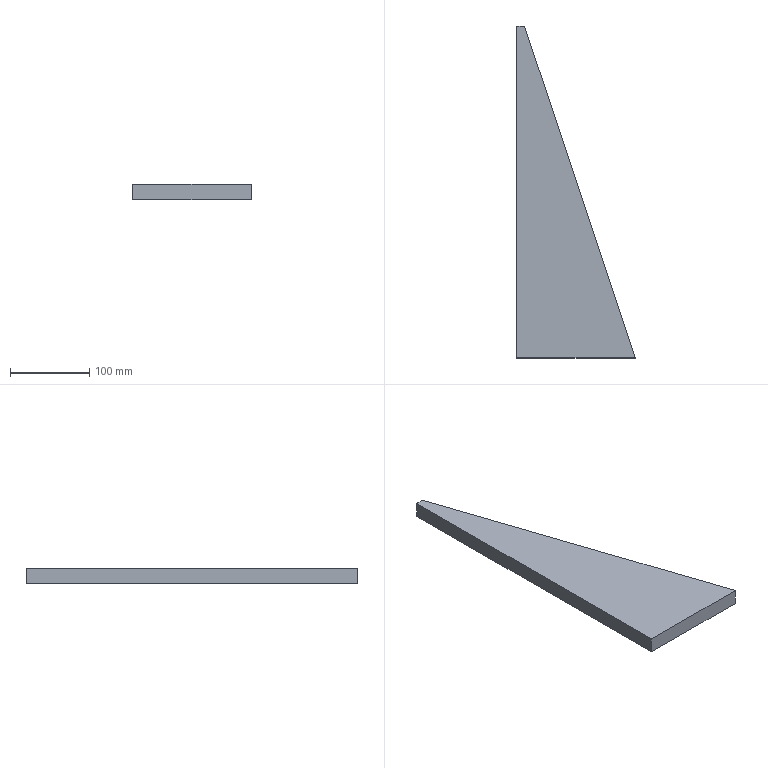Part | SolidWorks | features Extrusion 1 | 1 solid | 6 faces | box 150 x 420 x 20 mm | volume 672000 mm3 | plane 6
STEP:
#1=CARTESIAN_POINT('',(0.,420.,0.));
#2=VERTEX_POINT('',#1);
#3=CARTESIAN_POINT('',(0.,0.,0.));
#4=VERTEX_POINT('',#3);
#5=CARTESIAN_POINT('',(0.,0.,0.));
#6=DIRECTION('',(0.,-1.,0.));
#7=VECTOR('',#6,1000.);
#8=LINE('',#5,#7);
#9=EDGE_CURVE('',#2,#4,#8,.T.);
#10=ORIENTED_EDGE('',*,*,#9,.T.);
#11=CARTESIAN_POINT('',(0.,0.,20.));
#12=VERTEX_POINT('',#11);
#13=CARTESIAN_POINT('',(0.,0.,20.));
#14=DIRECTION('',(0.,0.,-1.));
#15=VECTOR('',#14,1000.);
#16=LINE('',#13,#15);
#17=EDGE_CURVE('',#12,#4,#16,.T.);
#18=ORIENTED_EDGE('',*,*,#17,.F.);
#19=CARTESIAN_POINT('',(0.,420.,20.));
#20=VERTEX_POINT('',#19);
#21=CARTESIAN_POINT('',(0.,0.,20.));
#22=DIRECTION('',(0.,-1.,0.));
#23=VECTOR('',#22,1000.);
#24=LINE('',#21,#23);
#25=EDGE_CURVE('',#20,#12,#24,.T.);
#26=ORIENTED_EDGE('',*,*,#25,.F.);
#27=CARTESIAN_POINT('',(0.,420.,20.));
#28=DIRECTION('',(0.,0.,-1.));
#29=VECTOR('',#28,1000.);
#30=LINE('',#27,#29);
#31=EDGE_CURVE('',#20,#2,#30,.T.);
#32=ORIENTED_EDGE('',*,*,#31,.T.);
#33=EDGE_LOOP('',(#10,#18,#26,#32));
#34=FACE_OUTER_BOUND('',#33,.T.);
#35=CARTESIAN_POINT('',(0.,0.,20.));
#36=DIRECTION('',(1.,0.,0.));
#37=DIRECTION('',(0.,0.,-1.));
#38=AXIS2_PLACEMENT_3D('',#35,#36,#37);
#39=PLANE('',#38);
#40=ADVANCED_FACE('',(#34),#39,.F.);
#41=CARTESIAN_POINT('',(150.,0.,0.));
#42=VERTEX_POINT('',#41);
#43=CARTESIAN_POINT('',(0.,0.,0.));
#44=DIRECTION('',(1.,0.,0.));
#45=VECTOR('',#44,1000.);
#46=LINE('',#43,#45);
#47=EDGE_CURVE('',#4,#42,#46,.T.);
#48=ORIENTED_EDGE('',*,*,#47,.T.);
#49=CARTESIAN_POINT('',(150.,0.,20.));
#50=VERTEX_POINT('',#49);
#51=CARTESIAN_POINT('',(150.,0.,20.));
#52=DIRECTION('',(0.,0.,-1.));
#53=VECTOR('',#52,1000.);
#54=LINE('',#51,#53);
#55=EDGE_CURVE('',#50,#42,#54,.T.);
#56=ORIENTED_EDGE('',*,*,#55,.F.);
#57=CARTESIAN_POINT('',(0.,0.,20.));
#58=DIRECTION('',(1.,0.,0.));
#59=VECTOR('',#58,1000.);
#60=LINE('',#57,#59);
#61=EDGE_CURVE('',#12,#50,#60,.T.);
#62=ORIENTED_EDGE('',*,*,#61,.F.);
#63=ORIENTED_EDGE('',*,*,#17,.T.);
#64=EDGE_LOOP('',(#48,#56,#62,#63));
#65=FACE_OUTER_BOUND('',#64,.T.);
#66=CARTESIAN_POINT('',(0.,0.,20.));
#67=DIRECTION('',(0.,1.,0.));
#68=DIRECTION('',(0.,0.,1.));
#69=AXIS2_PLACEMENT_3D('',#66,#67,#68);
#70=PLANE('',#69);
#71=ADVANCED_FACE('',(#65),#70,.F.);
#72=CARTESIAN_POINT('',(10.,420.,0.));
#73=VERTEX_POINT('',#72);
#74=CARTESIAN_POINT('',(10.,420.,0.));
#75=DIRECTION('',(-0.3162,0.9487,0.));
#76=VECTOR('',#75,1000.);
#77=LINE('',#74,#76);
#78=EDGE_CURVE('',#42,#73,#77,.T.);
#79=ORIENTED_EDGE('',*,*,#78,.T.);
#80=CARTESIAN_POINT('',(10.,420.,20.));
#81=VERTEX_POINT('',#80);
#82=CARTESIAN_POINT('',(10.,420.,20.));
#83=DIRECTION('',(0.,0.,-1.));
#84=VECTOR('',#83,1000.);
#85=LINE('',#82,#84);
#86=EDGE_CURVE('',#81,#73,#85,.T.);
#87=ORIENTED_EDGE('',*,*,#86,.F.);
#88=CARTESIAN_POINT('',(10.,420.,20.));
#89=DIRECTION('',(-0.3162,0.9487,0.));
#90=VECTOR('',#89,1000.);
#91=LINE('',#88,#90);
#92=EDGE_CURVE('',#50,#81,#91,.T.);
#93=ORIENTED_EDGE('',*,*,#92,.F.);
#94=ORIENTED_EDGE('',*,*,#55,.T.);
#95=EDGE_LOOP('',(#79,#87,#93,#94));
#96=FACE_OUTER_BOUND('',#95,.T.);
#97=CARTESIAN_POINT('',(10.,420.,20.));
#98=DIRECTION('',(-0.9487,-0.3162,0.));
#99=DIRECTION('',(0.3162,-0.9487,0.));
#100=AXIS2_PLACEMENT_3D('',#97,#98,#99);
#101=PLANE('',#100);
#102=ADVANCED_FACE('',(#96),#101,.F.);
#103=CARTESIAN_POINT('',(0.,420.,0.));
#104=DIRECTION('',(-1.,0.,0.));
#105=VECTOR('',#104,1000.);
#106=LINE('',#103,#105);
#107=EDGE_CURVE('',#73,#2,#106,.T.);
#108=ORIENTED_EDGE('',*,*,#107,.T.);
#109=ORIENTED_EDGE('',*,*,#31,.F.);
#110=CARTESIAN_POINT('',(0.,420.,20.));
#111=DIRECTION('',(-1.,0.,0.));
#112=VECTOR('',#111,1000.);
#113=LINE('',#110,#112);
#114=EDGE_CURVE('',#81,#20,#113,.T.);
#115=ORIENTED_EDGE('',*,*,#114,.F.);
#116=ORIENTED_EDGE('',*,*,#86,.T.);
#117=EDGE_LOOP('',(#108,#109,#115,#116));
#118=FACE_OUTER_BOUND('',#117,.T.);
#119=CARTESIAN_POINT('',(0.,420.,20.));
#120=DIRECTION('',(0.,-1.,0.));
#121=DIRECTION('',(0.,0.,-1.));
#122=AXIS2_PLACEMENT_3D('',#119,#120,#121);
#123=PLANE('',#122);
#124=ADVANCED_FACE('',(#118),#123,.F.);
#125=ORIENTED_EDGE('',*,*,#25,.T.);
#126=ORIENTED_EDGE('',*,*,#61,.T.);
#127=ORIENTED_EDGE('',*,*,#92,.T.);
#128=ORIENTED_EDGE('',*,*,#114,.T.);
#129=EDGE_LOOP('',(#125,#126,#127,#128));
#130=FACE_OUTER_BOUND('',#129,.T.);
#131=CARTESIAN_POINT('',(0.,0.,20.));
#132=DIRECTION('',(0.,0.,-1.));
#133=DIRECTION('',(-1.,0.,0.));
#134=AXIS2_PLACEMENT_3D('',#131,#132,#133);
#135=PLANE('',#134);
#136=ADVANCED_FACE('',(#130),#135,.F.);
#137=ORIENTED_EDGE('',*,*,#9,.F.);
#138=ORIENTED_EDGE('',*,*,#107,.F.);
#139=ORIENTED_EDGE('',*,*,#78,.F.);
#140=ORIENTED_EDGE('',*,*,#47,.F.);
#141=EDGE_LOOP('',(#137,#138,#139,#140));
#142=FACE_OUTER_BOUND('',#141,.T.);
#143=CARTESIAN_POINT('',(0.,0.,0.));
#144=DIRECTION('',(0.,0.,-1.));
#145=DIRECTION('',(-1.,0.,0.));
#146=AXIS2_PLACEMENT_3D('',#143,#144,#145);
#147=PLANE('',#146);
#148=ADVANCED_FACE('',(#142),#147,.T.);
#149=CLOSED_SHELL('',(#40,#71,#102,#124,#136,#148));
#150=MANIFOLD_SOLID_BREP('',#149);
#151=CARTESIAN_POINT('',(0.,0.,0.));
#152=DIRECTION('',(0.,0.,1.));
#153=DIRECTION('',(1.,0.,0.));
#154=AXIS2_PLACEMENT_3D('',#151,#152,#153);
#155=(LENGTH_UNIT()NAMED_UNIT(*)SI_UNIT(.MILLI.,.METRE.));
#156=UNCERTAINTY_MEASURE_WITH_UNIT(LENGTH_MEASURE(0.00001),#155,'','');
#157=(NAMED_UNIT(*)PLANE_ANGLE_UNIT()SI_UNIT($,.RADIAN.));
#158=(NAMED_UNIT(*)SI_UNIT($,.STERADIAN.)SOLID_ANGLE_UNIT());
#159=(GEOMETRIC_REPRESENTATION_CONTEXT(3)GLOBAL_UNCERTAINTY_ASSIGNED_CONTEXT((#156))GLOBAL_UNIT_ASSIGNED_CONTEXT((#155,#157,#158))REPRESENTATION_CONTEXT('',''));
#160=ADVANCED_BREP_SHAPE_REPRESENTATION('',(#150,#154),#159);